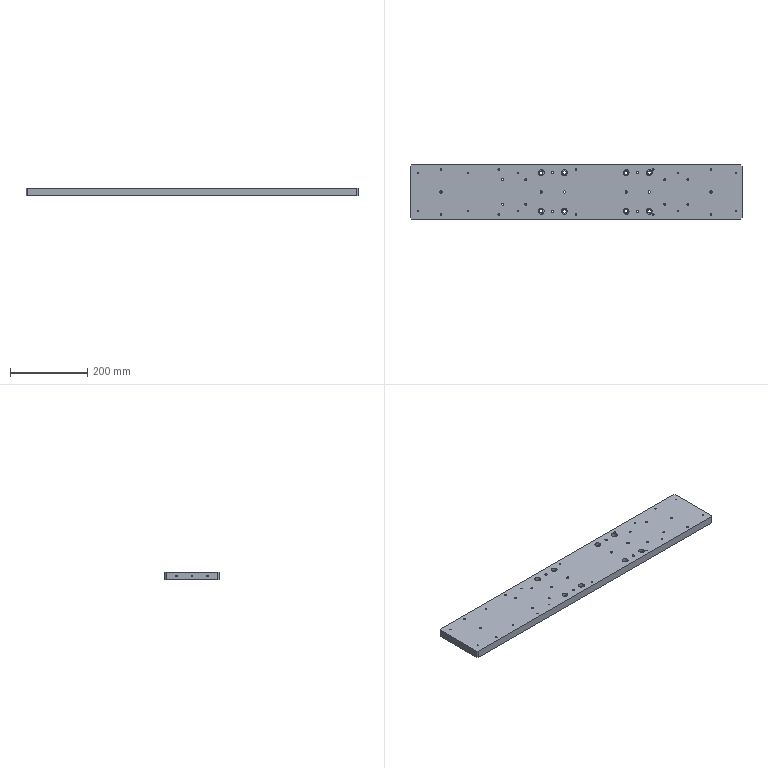Part | 1 solid | 84 faces | box 860 x 140 x 20 mm | volume 2375336 mm3 | cylinder 60 | plane 18 | cone 6 | commonest cylinder face diameters 4.2 x16 3.3 x10 6 x10 5 x8 9 x8 15 x8